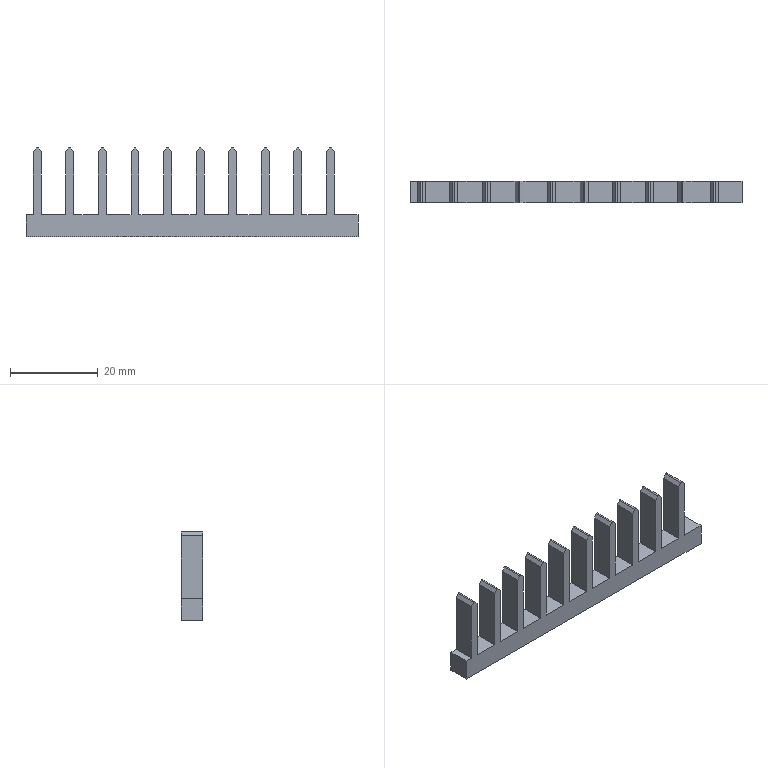Part | STEP file | 200 mesh_id1870 | 1 solid | 66 faces | box 75.6 x 4.94 x 20.309 mm | volume 3191 mm3 | plane 56 | cylinder 10 | commonest cylinder face diameters 0.5 x10